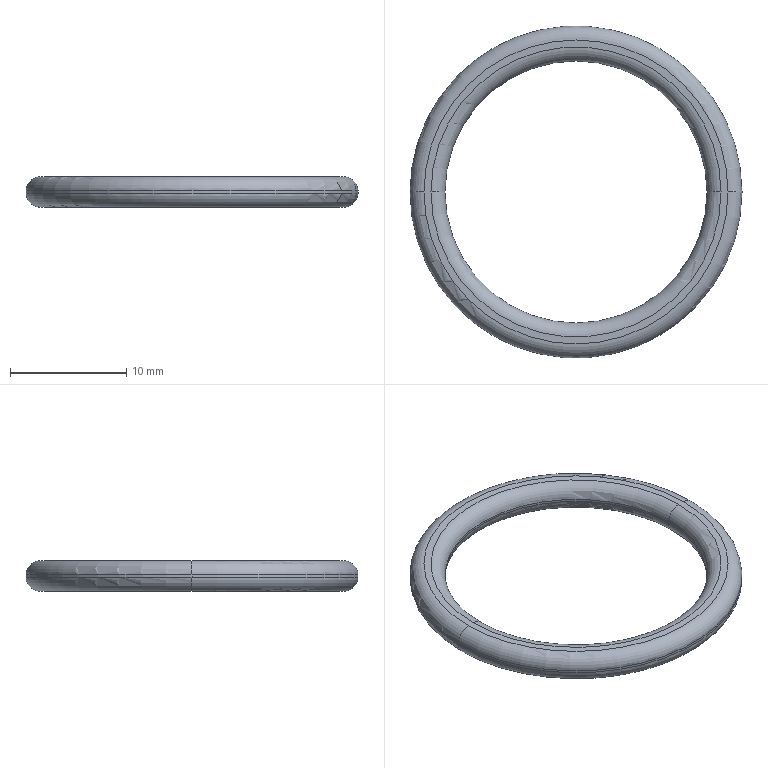Part | STEP file | MIFENGQUAN2 | 1 solid | 14 faces | box 28.5 x 28.5 x 2.6 mm | volume 525.838 mm3 | torus 8 | cylinder 4 | plane 2 | commonest cylinder face diameters 22.5 x2 28.5 x2
STEP:
#1=CARTESIAN_POINT('',(0.,0.,0.));
#2=DIRECTION('',(0.,0.,1.));
#3=DIRECTION('',(1.,0.,0.));
#4=AXIS2_PLACEMENT_3D('',#1,#2,#3);
#5=CARTESIAN_POINT('',(-14.25,0.,-0.1));
#6=VERTEX_POINT('',#5);
#7=CARTESIAN_POINT('',(14.25,0.,-0.1));
#8=VERTEX_POINT('',#7);
#9=CARTESIAN_POINT('',(0.,0.,-0.1));
#10=DIRECTION('',(0.,0.,1.));
#11=DIRECTION('',(-1.,0.,0.));
#12=AXIS2_PLACEMENT_3D('',#9,#10,#11);
#13=CIRCLE('',#12,14.25);
#14=EDGE_CURVE('',#6,#8,#13,.T.);
#15=ORIENTED_EDGE('',*,*,#14,.F.);
#16=CARTESIAN_POINT('',(-14.25,0.,0.1));
#17=VERTEX_POINT('',#16);
#18=CARTESIAN_POINT('',(-14.25,0.,-0.1));
#19=DIRECTION('',(0.,0.,1.));
#20=VECTOR('',#19,0.2);
#21=LINE('',#18,#20);
#22=EDGE_CURVE('',#6,#17,#21,.T.);
#23=ORIENTED_EDGE('',*,*,#22,.T.);
#24=CARTESIAN_POINT('',(14.25,0.,0.1));
#25=VERTEX_POINT('',#24);
#26=CARTESIAN_POINT('',(0.,0.,0.1));
#27=DIRECTION('',(0.,0.,1.));
#28=DIRECTION('',(-1.,0.,0.));
#29=AXIS2_PLACEMENT_3D('',#26,#27,#28);
#30=CIRCLE('',#29,14.25);
#31=EDGE_CURVE('',#17,#25,#30,.T.);
#32=ORIENTED_EDGE('',*,*,#31,.T.);
#33=CARTESIAN_POINT('',(14.25,0.,-0.1));
#34=DIRECTION('',(0.,0.,1.));
#35=VECTOR('',#34,0.2);
#36=LINE('',#33,#35);
#37=EDGE_CURVE('',#8,#25,#36,.T.);
#38=ORIENTED_EDGE('',*,*,#37,.F.);
#39=EDGE_LOOP('',(#15,#23,#32,#38));
#40=FACE_OUTER_BOUND('',#39,.F.);
#41=CARTESIAN_POINT('',(0.,0.,-1.43));
#42=DIRECTION('',(0.,0.,1.));
#43=DIRECTION('',(-1.,0.,0.));
#44=AXIS2_PLACEMENT_3D('',#41,#42,#43);
#45=CYLINDRICAL_SURFACE('',#44,14.25);
#46=ADVANCED_FACE('',(#40),#45,.T.);
#47=ORIENTED_EDGE('',*,*,#14,.T.);
#48=CARTESIAN_POINT('',(13.05,0.,-1.3));
#49=VERTEX_POINT('',#48);
#50=CARTESIAN_POINT('',(13.05,0.,-0.1));
#51=DIRECTION('',(0.,1.,0.));
#52=DIRECTION('',(1.,0.,0.));
#53=AXIS2_PLACEMENT_3D('',#50,#51,#52);
#54=CIRCLE('',#53,1.2);
#55=EDGE_CURVE('',#8,#49,#54,.T.);
#56=ORIENTED_EDGE('',*,*,#55,.T.);
#57=CARTESIAN_POINT('',(-13.05,0.,-1.3));
#58=VERTEX_POINT('',#57);
#59=CARTESIAN_POINT('',(0.,0.,-1.3));
#60=DIRECTION('',(0.,0.,1.));
#61=DIRECTION('',(-1.,0.,0.));
#62=AXIS2_PLACEMENT_3D('',#59,#60,#61);
#63=CIRCLE('',#62,13.05);
#64=EDGE_CURVE('',#58,#49,#63,.T.);
#65=ORIENTED_EDGE('',*,*,#64,.F.);
#66=CARTESIAN_POINT('',(-13.05,0.,-0.1));
#67=DIRECTION('',(0.,-1.,0.));
#68=DIRECTION('',(-1.,0.,0.));
#69=AXIS2_PLACEMENT_3D('',#66,#67,#68);
#70=CIRCLE('',#69,1.2);
#71=EDGE_CURVE('',#6,#58,#70,.T.);
#72=ORIENTED_EDGE('',*,*,#71,.F.);
#73=EDGE_LOOP('',(#47,#56,#65,#72));
#74=FACE_OUTER_BOUND('',#73,.F.);
#75=CARTESIAN_POINT('',(0.,0.,-0.1));
#76=DIRECTION('',(0.,0.,1.));
#77=DIRECTION('',(-1.,0.004568,0.));
#78=AXIS2_PLACEMENT_3D('',#75,#76,#77);
#79=TOROIDAL_SURFACE('',#78,13.05,1.2);
#80=ADVANCED_FACE('',(#74),#79,.T.);
#81=CARTESIAN_POINT('',(0.,0.,-0.1));
#82=DIRECTION('',(0.,0.,1.));
#83=DIRECTION('',(1.,0.,0.));
#84=AXIS2_PLACEMENT_3D('',#81,#82,#83);
#85=CIRCLE('',#84,14.25);
#86=EDGE_CURVE('',#8,#6,#85,.T.);
#87=ORIENTED_EDGE('',*,*,#86,.T.);
#88=ORIENTED_EDGE('',*,*,#71,.T.);
#89=CARTESIAN_POINT('',(0.,0.,-1.3));
#90=DIRECTION('',(0.,0.,1.));
#91=DIRECTION('',(1.,0.,0.));
#92=AXIS2_PLACEMENT_3D('',#89,#90,#91);
#93=CIRCLE('',#92,13.05);
#94=EDGE_CURVE('',#49,#58,#93,.T.);
#95=ORIENTED_EDGE('',*,*,#94,.F.);
#96=ORIENTED_EDGE('',*,*,#55,.F.);
#97=EDGE_LOOP('',(#87,#88,#95,#96));
#98=FACE_OUTER_BOUND('',#97,.F.);
#99=CARTESIAN_POINT('',(0.,0.,-0.1));
#100=DIRECTION('',(0.,0.,1.));
#101=DIRECTION('',(1.,-0.004568,0.));
#102=AXIS2_PLACEMENT_3D('',#99,#100,#101);
#103=TOROIDAL_SURFACE('',#102,13.05,1.2);
#104=ADVANCED_FACE('',(#98),#103,.T.);
#105=ORIENTED_EDGE('',*,*,#86,.F.);
#106=ORIENTED_EDGE('',*,*,#37,.T.);
#107=CARTESIAN_POINT('',(0.,0.,0.1));
#108=DIRECTION('',(0.,0.,1.));
#109=DIRECTION('',(1.,0.,0.));
#110=AXIS2_PLACEMENT_3D('',#107,#108,#109);
#111=CIRCLE('',#110,14.25);
#112=EDGE_CURVE('',#25,#17,#111,.T.);
#113=ORIENTED_EDGE('',*,*,#112,.T.);
#114=ORIENTED_EDGE('',*,*,#22,.F.);
#115=EDGE_LOOP('',(#105,#106,#113,#114));
#116=FACE_OUTER_BOUND('',#115,.F.);
#117=CARTESIAN_POINT('',(0.,0.,-1.43));
#118=DIRECTION('',(0.,0.,1.));
#119=DIRECTION('',(-1.,0.,0.));
#120=AXIS2_PLACEMENT_3D('',#117,#118,#119);
#121=CYLINDRICAL_SURFACE('',#120,14.25);
#122=ADVANCED_FACE('',(#116),#121,.T.);
#123=CARTESIAN_POINT('',(13.05,0.,1.3));
#124=VERTEX_POINT('',#123);
#125=CARTESIAN_POINT('',(-13.05,0.,1.3));
#126=VERTEX_POINT('',#125);
#127=CARTESIAN_POINT('',(0.,0.,1.3));
#128=DIRECTION('',(0.,0.,1.));
#129=DIRECTION('',(1.,0.,0.));
#130=AXIS2_PLACEMENT_3D('',#127,#128,#129);
#131=CIRCLE('',#130,13.05);
#132=EDGE_CURVE('',#124,#126,#131,.T.);
#133=ORIENTED_EDGE('',*,*,#132,.T.);
#134=CARTESIAN_POINT('',(-13.05,0.,0.1));
#135=DIRECTION('',(0.,-1.,0.));
#136=DIRECTION('',(0.,0.,1.));
#137=AXIS2_PLACEMENT_3D('',#134,#135,#136);
#138=CIRCLE('',#137,1.2);
#139=EDGE_CURVE('',#126,#17,#138,.T.);
#140=ORIENTED_EDGE('',*,*,#139,.T.);
#141=ORIENTED_EDGE('',*,*,#112,.F.);
#142=CARTESIAN_POINT('',(13.05,0.,0.1));
#143=DIRECTION('',(0.,1.,0.));
#144=DIRECTION('',(0.,0.,1.));
#145=AXIS2_PLACEMENT_3D('',#142,#143,#144);
#146=CIRCLE('',#145,1.2);
#147=EDGE_CURVE('',#124,#25,#146,.T.);
#148=ORIENTED_EDGE('',*,*,#147,.F.);
#149=EDGE_LOOP('',(#133,#140,#141,#148));
#150=FACE_OUTER_BOUND('',#149,.F.);
#151=CARTESIAN_POINT('',(0.,0.,0.1));
#152=DIRECTION('',(0.,0.,1.));
#153=DIRECTION('',(1.,-0.004358,0.));
#154=AXIS2_PLACEMENT_3D('',#151,#152,#153);
#155=TOROIDAL_SURFACE('',#154,13.05,1.2);
#156=ADVANCED_FACE('',(#150),#155,.T.);
#157=CARTESIAN_POINT('',(0.,0.,1.3));
#158=DIRECTION('',(0.,0.,1.));
#159=DIRECTION('',(-1.,0.,0.));
#160=AXIS2_PLACEMENT_3D('',#157,#158,#159);
#161=CIRCLE('',#160,13.05);
#162=EDGE_CURVE('',#126,#124,#161,.T.);
#163=ORIENTED_EDGE('',*,*,#162,.F.);
#164=ORIENTED_EDGE('',*,*,#132,.F.);
#165=EDGE_LOOP('',(#163,#164));
#166=FACE_OUTER_BOUND('',#165,.F.);
#167=CARTESIAN_POINT('',(12.45,0.,1.3));
#168=VERTEX_POINT('',#167);
#169=CARTESIAN_POINT('',(-12.45,0.,1.3));
#170=VERTEX_POINT('',#169);
#171=CARTESIAN_POINT('',(0.,0.,1.3));
#172=DIRECTION('',(0.,0.,1.));
#173=DIRECTION('',(1.,0.,0.));
#174=AXIS2_PLACEMENT_3D('',#171,#172,#173);
#175=CIRCLE('',#174,12.45);
#176=EDGE_CURVE('',#168,#170,#175,.T.);
#177=ORIENTED_EDGE('',*,*,#176,.T.);
#178=CARTESIAN_POINT('',(0.,0.,1.3));
#179=DIRECTION('',(0.,0.,1.));
#180=DIRECTION('',(-1.,0.,0.));
#181=AXIS2_PLACEMENT_3D('',#178,#179,#180);
#182=CIRCLE('',#181,12.45);
#183=EDGE_CURVE('',#170,#168,#182,.T.);
#184=ORIENTED_EDGE('',*,*,#183,.T.);
#185=EDGE_LOOP('',(#177,#184));
#186=FACE_BOUND('',#185,.F.);
#187=CARTESIAN_POINT('',(0.,0.,1.3));
#188=DIRECTION('',(0.,0.,1.));
#189=DIRECTION('',(-1.,0.,0.));
#190=AXIS2_PLACEMENT_3D('',#187,#188,#189);
#191=PLANE('',#190);
#192=ADVANCED_FACE('',(#166,#186),#191,.T.);
#193=ORIENTED_EDGE('',*,*,#162,.T.);
#194=ORIENTED_EDGE('',*,*,#147,.T.);
#195=ORIENTED_EDGE('',*,*,#31,.F.);
#196=ORIENTED_EDGE('',*,*,#139,.F.);
#197=EDGE_LOOP('',(#193,#194,#195,#196));
#198=FACE_OUTER_BOUND('',#197,.F.);
#199=CARTESIAN_POINT('',(0.,0.,0.1));
#200=DIRECTION('',(0.,0.,1.));
#201=DIRECTION('',(-1.,0.004358,0.));
#202=AXIS2_PLACEMENT_3D('',#199,#200,#201);
#203=TOROIDAL_SURFACE('',#202,13.05,1.2);
#204=ADVANCED_FACE('',(#198),#203,.T.);
#205=CARTESIAN_POINT('',(11.25,0.,0.1));
#206=VERTEX_POINT('',#205);
#207=CARTESIAN_POINT('',(-11.25,0.,0.1));
#208=VERTEX_POINT('',#207);
#209=CARTESIAN_POINT('',(0.,0.,0.1));
#210=DIRECTION('',(0.,0.,1.));
#211=DIRECTION('',(1.,0.,0.));
#212=AXIS2_PLACEMENT_3D('',#209,#210,#211);
#213=CIRCLE('',#212,11.25);
#214=EDGE_CURVE('',#206,#208,#213,.T.);
#215=ORIENTED_EDGE('',*,*,#214,.T.);
#216=CARTESIAN_POINT('',(-12.45,0.,0.1));
#217=DIRECTION('',(0.,-1.,0.));
#218=DIRECTION('',(1.,0.,0.));
#219=AXIS2_PLACEMENT_3D('',#216,#217,#218);
#220=CIRCLE('',#219,1.2);
#221=EDGE_CURVE('',#208,#170,#220,.T.);
#222=ORIENTED_EDGE('',*,*,#221,.T.);
#223=ORIENTED_EDGE('',*,*,#176,.F.);
#224=CARTESIAN_POINT('',(12.45,0.,0.1));
#225=DIRECTION('',(0.,1.,0.));
#226=DIRECTION('',(-1.,0.,0.));
#227=AXIS2_PLACEMENT_3D('',#224,#225,#226);
#228=CIRCLE('',#227,1.2);
#229=EDGE_CURVE('',#206,#168,#228,.T.);
#230=ORIENTED_EDGE('',*,*,#229,.F.);
#231=EDGE_LOOP('',(#215,#222,#223,#230));
#232=FACE_OUTER_BOUND('',#231,.F.);
#233=CARTESIAN_POINT('',(0.,0.,0.1));
#234=DIRECTION('',(0.,0.,1.));
#235=DIRECTION('',(1.,-0.005786,0.));
#236=AXIS2_PLACEMENT_3D('',#233,#234,#235);
#237=TOROIDAL_SURFACE('',#236,12.45,1.2);
#238=ADVANCED_FACE('',(#232),#237,.T.);
#239=CARTESIAN_POINT('',(11.25,0.,-0.1));
#240=VERTEX_POINT('',#239);
#241=CARTESIAN_POINT('',(-11.25,0.,-0.1));
#242=VERTEX_POINT('',#241);
#243=CARTESIAN_POINT('',(0.,0.,-0.1));
#244=DIRECTION('',(0.,0.,1.));
#245=DIRECTION('',(1.,0.,0.));
#246=AXIS2_PLACEMENT_3D('',#243,#244,#245);
#247=CIRCLE('',#246,11.25);
#248=EDGE_CURVE('',#240,#242,#247,.T.);
#249=ORIENTED_EDGE('',*,*,#248,.T.);
#250=CARTESIAN_POINT('',(-11.25,0.,0.1));
#251=DIRECTION('',(0.,0.,-1.));
#252=VECTOR('',#251,0.2);
#253=LINE('',#250,#252);
#254=EDGE_CURVE('',#208,#242,#253,.T.);
#255=ORIENTED_EDGE('',*,*,#254,.F.);
#256=ORIENTED_EDGE('',*,*,#214,.F.);
#257=CARTESIAN_POINT('',(11.25,0.,0.1));
#258=DIRECTION('',(0.,0.,-1.));
#259=VECTOR('',#258,0.2);
#260=LINE('',#257,#259);
#261=EDGE_CURVE('',#206,#240,#260,.T.);
#262=ORIENTED_EDGE('',*,*,#261,.T.);
#263=EDGE_LOOP('',(#249,#255,#256,#262));
#264=FACE_OUTER_BOUND('',#263,.F.);
#265=CARTESIAN_POINT('',(0.,0.,-1.43));
#266=DIRECTION('',(0.,0.,1.));
#267=DIRECTION('',(-1.,0.,0.));
#268=AXIS2_PLACEMENT_3D('',#265,#266,#267);
#269=CYLINDRICAL_SURFACE('',#268,11.25);
#270=ADVANCED_FACE('',(#264),#269,.F.);
#271=CARTESIAN_POINT('',(12.45,0.,-1.3));
#272=VERTEX_POINT('',#271);
#273=CARTESIAN_POINT('',(-12.45,0.,-1.3));
#274=VERTEX_POINT('',#273);
#275=CARTESIAN_POINT('',(0.,0.,-1.3));
#276=DIRECTION('',(0.,0.,1.));
#277=DIRECTION('',(1.,0.,0.));
#278=AXIS2_PLACEMENT_3D('',#275,#276,#277);
#279=CIRCLE('',#278,12.45);
#280=EDGE_CURVE('',#272,#274,#279,.T.);
#281=ORIENTED_EDGE('',*,*,#280,.T.);
#282=CARTESIAN_POINT('',(-12.45,0.,-0.1));
#283=DIRECTION('',(0.,-1.,0.));
#284=DIRECTION('',(0.,0.,-1.));
#285=AXIS2_PLACEMENT_3D('',#282,#283,#284);
#286=CIRCLE('',#285,1.2);
#287=EDGE_CURVE('',#274,#242,#286,.T.);
#288=ORIENTED_EDGE('',*,*,#287,.T.);
#289=ORIENTED_EDGE('',*,*,#248,.F.);
#290=CARTESIAN_POINT('',(12.45,0.,-0.1));
#291=DIRECTION('',(0.,1.,0.));
#292=DIRECTION('',(0.,0.,-1.));
#293=AXIS2_PLACEMENT_3D('',#290,#291,#292);
#294=CIRCLE('',#293,1.2);
#295=EDGE_CURVE('',#272,#240,#294,.T.);
#296=ORIENTED_EDGE('',*,*,#295,.F.);
#297=EDGE_LOOP('',(#281,#288,#289,#296));
#298=FACE_OUTER_BOUND('',#297,.F.);
#299=CARTESIAN_POINT('',(0.,0.,-0.1));
#300=DIRECTION('',(0.,0.,1.));
#301=DIRECTION('',(1.,-0.00552,0.));
#302=AXIS2_PLACEMENT_3D('',#299,#300,#301);
#303=TOROIDAL_SURFACE('',#302,12.45,1.2);
#304=ADVANCED_FACE('',(#298),#303,.T.);
#305=ORIENTED_EDGE('',*,*,#94,.T.);
#306=ORIENTED_EDGE('',*,*,#64,.T.);
#307=EDGE_LOOP('',(#305,#306));
#308=FACE_OUTER_BOUND('',#307,.F.);
#309=ORIENTED_EDGE('',*,*,#280,.F.);
#310=CARTESIAN_POINT('',(0.,0.,-1.3));
#311=DIRECTION('',(0.,0.,1.));
#312=DIRECTION('',(-1.,0.,0.));
#313=AXIS2_PLACEMENT_3D('',#310,#311,#312);
#314=CIRCLE('',#313,12.45);
#315=EDGE_CURVE('',#274,#272,#314,.T.);
#316=ORIENTED_EDGE('',*,*,#315,.F.);
#317=EDGE_LOOP('',(#309,#316));
#318=FACE_BOUND('',#317,.F.);
#319=CARTESIAN_POINT('',(0.,0.,-1.3));
#320=DIRECTION('',(0.,0.,1.));
#321=DIRECTION('',(-1.,0.,0.));
#322=AXIS2_PLACEMENT_3D('',#319,#320,#321);
#323=PLANE('',#322);
#324=ADVANCED_FACE('',(#308,#318),#323,.F.);
#325=ORIENTED_EDGE('',*,*,#315,.T.);
#326=ORIENTED_EDGE('',*,*,#295,.T.);
#327=CARTESIAN_POINT('',(0.,0.,-0.1));
#328=DIRECTION('',(0.,0.,1.));
#329=DIRECTION('',(-1.,0.,0.));
#330=AXIS2_PLACEMENT_3D('',#327,#328,#329);
#331=CIRCLE('',#330,11.25);
#332=EDGE_CURVE('',#242,#240,#331,.T.);
#333=ORIENTED_EDGE('',*,*,#332,.F.);
#334=ORIENTED_EDGE('',*,*,#287,.F.);
#335=EDGE_LOOP('',(#325,#326,#333,#334));
#336=FACE_OUTER_BOUND('',#335,.F.);
#337=CARTESIAN_POINT('',(0.,0.,-0.1));
#338=DIRECTION('',(0.,0.,1.));
#339=DIRECTION('',(-1.,0.00552,0.));
#340=AXIS2_PLACEMENT_3D('',#337,#338,#339);
#341=TOROIDAL_SURFACE('',#340,12.45,1.2);
#342=ADVANCED_FACE('',(#336),#341,.T.);
#343=ORIENTED_EDGE('',*,*,#332,.T.);
#344=ORIENTED_EDGE('',*,*,#261,.F.);
#345=CARTESIAN_POINT('',(0.,0.,0.1));
#346=DIRECTION('',(0.,0.,1.));
#347=DIRECTION('',(-1.,0.,0.));
#348=AXIS2_PLACEMENT_3D('',#345,#346,#347);
#349=CIRCLE('',#348,11.25);
#350=EDGE_CURVE('',#208,#206,#349,.T.);
#351=ORIENTED_EDGE('',*,*,#350,.F.);
#352=ORIENTED_EDGE('',*,*,#254,.T.);
#353=EDGE_LOOP('',(#343,#344,#351,#352));
#354=FACE_OUTER_BOUND('',#353,.F.);
#355=CARTESIAN_POINT('',(0.,0.,-1.43));
#356=DIRECTION('',(0.,0.,1.));
#357=DIRECTION('',(-1.,0.,0.));
#358=AXIS2_PLACEMENT_3D('',#355,#356,#357);
#359=CYLINDRICAL_SURFACE('',#358,11.25);
#360=ADVANCED_FACE('',(#354),#359,.F.);
#361=ORIENTED_EDGE('',*,*,#350,.T.);
#362=ORIENTED_EDGE('',*,*,#229,.T.);
#363=ORIENTED_EDGE('',*,*,#183,.F.);
#364=ORIENTED_EDGE('',*,*,#221,.F.);
#365=EDGE_LOOP('',(#361,#362,#363,#364));
#366=FACE_OUTER_BOUND('',#365,.F.);
#367=CARTESIAN_POINT('',(0.,0.,0.1));
#368=DIRECTION('',(0.,0.,1.));
#369=DIRECTION('',(-1.,0.005786,0.));
#370=AXIS2_PLACEMENT_3D('',#367,#368,#369);
#371=TOROIDAL_SURFACE('',#370,12.45,1.2);
#372=ADVANCED_FACE('',(#366),#371,.T.);
#373=CLOSED_SHELL('',(#46,#80,#104,#122,#156,#192,#204,#238,#270,#304,#324,#342,#360,#372));
#374=MANIFOLD_SOLID_BREP('',#373);
#375=(LENGTH_UNIT()NAMED_UNIT(*)SI_UNIT(.MILLI.,.METRE.));
#376=UNCERTAINTY_MEASURE_WITH_UNIT(LENGTH_MEASURE(0.004039),#375,'','');
#377=(NAMED_UNIT(*)PLANE_ANGLE_UNIT()SI_UNIT($,.RADIAN.));
#378=PLANE_ANGLE_MEASURE_WITH_UNIT(PLANE_ANGLE_MEASURE(0.01745),#377);
#379=(CONVERSION_BASED_UNIT('DEGREE',#378)NAMED_UNIT(*)PLANE_ANGLE_UNIT());
#380=(NAMED_UNIT(*)SI_UNIT($,.STERADIAN.)SOLID_ANGLE_UNIT());
#381=(GEOMETRIC_REPRESENTATION_CONTEXT(3)GLOBAL_UNCERTAINTY_ASSIGNED_CONTEXT((#376))GLOBAL_UNIT_ASSIGNED_CONTEXT((#375,#379,#380))REPRESENTATION_CONTEXT('',''));
#382=ADVANCED_BREP_SHAPE_REPRESENTATION('',(#4,#374),#381);